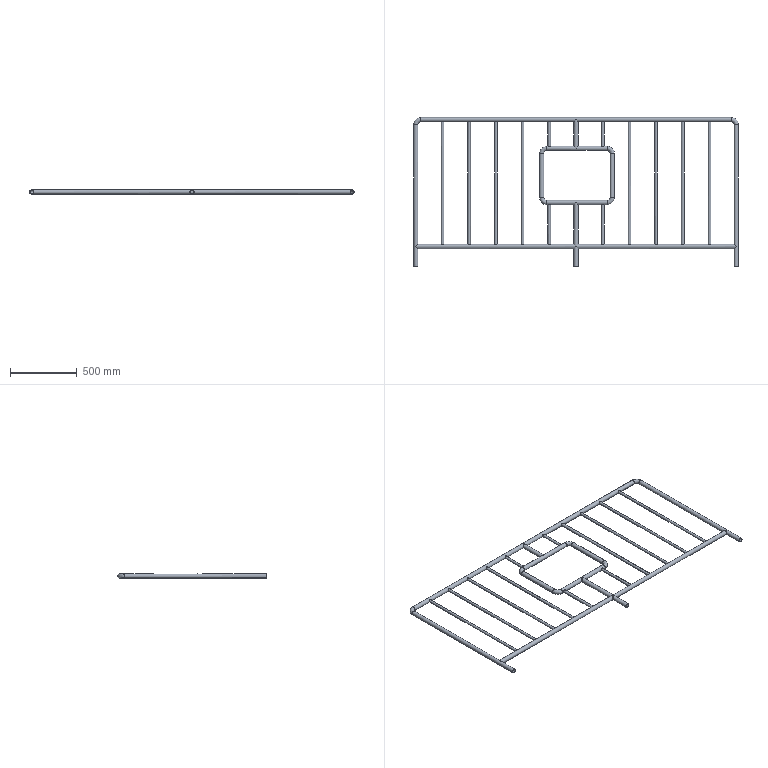Part | STEP file | PN_0057 304 guardrail 2400X1100 body A_Default<As Machined> | 22 solids | 100 faces | box 2432 x 1116 x 32 mm | volume 2712212 mm3 | cylinder 77 | torus 12 | plane 11 | commonest cylinder face diameters 32 x42 16 x12 20 x12 28 x11